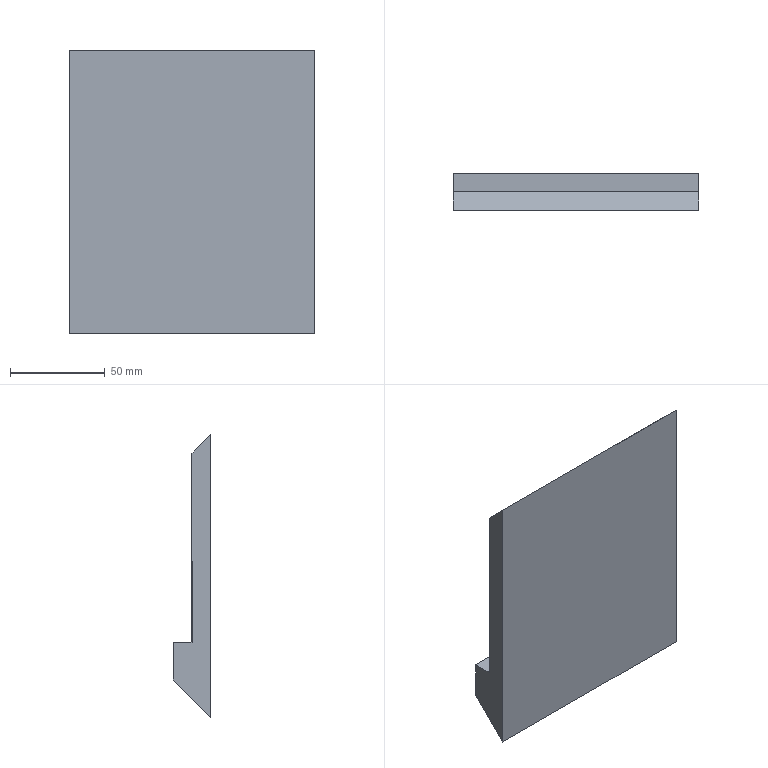Part | NX | features solid 2 | 1 solid | 8 faces | box 130 x 20 x 150 mm | volume 214500 mm3 | plane 8
STEP:
#1=CARTESIAN_POINT('',(830.,185.,120.));
#2=VERTEX_POINT('',#1);
#3=CARTESIAN_POINT('',(700.,185.,120.));
#4=VERTEX_POINT('',#3);
#5=CARTESIAN_POINT('',(695.,185.,120.));
#6=DIRECTION('',(1.,0.,0.));
#7=VECTOR('',#6,1000.);
#8=LINE('',#5,#7);
#9=EDGE_CURVE('',#2,#4,#8,.F.);
#10=ORIENTED_EDGE('',*,*,#9,.F.);
#11=CARTESIAN_POINT('',(830.,185.,20.));
#12=VERTEX_POINT('',#11);
#13=CARTESIAN_POINT('',(830.,185.,10.));
#14=DIRECTION('',(0.,0.,1.));
#15=VECTOR('',#14,1000.);
#16=LINE('',#13,#15);
#17=EDGE_CURVE('',#12,#2,#16,.T.);
#18=ORIENTED_EDGE('',*,*,#17,.F.);
#19=CARTESIAN_POINT('',(700.,185.,20.));
#20=VERTEX_POINT('',#19);
#21=CARTESIAN_POINT('',(730.,185.,20.));
#22=DIRECTION('',(1.,0.,0.));
#23=VECTOR('',#22,1000.);
#24=LINE('',#21,#23);
#25=EDGE_CURVE('',#20,#12,#24,.T.);
#26=ORIENTED_EDGE('',*,*,#25,.F.);
#27=CARTESIAN_POINT('',(700.,185.,95.));
#28=DIRECTION('',(0.,0.,-1.));
#29=VECTOR('',#28,1000.);
#30=LINE('',#27,#29);
#31=EDGE_CURVE('',#4,#20,#30,.T.);
#32=ORIENTED_EDGE('',*,*,#31,.F.);
#33=EDGE_LOOP('',(#10,#18,#26,#32));
#34=FACE_BOUND('',#33,.T.);
#35=CARTESIAN_POINT('',(730.,185.,10.));
#36=DIRECTION('',(0.,1.,0.));
#37=DIRECTION('',(1.,0.,0.));
#38=AXIS2_PLACEMENT_3D('',#35,#36,#37);
#39=PLANE('',#38);
#40=ADVANCED_FACE('',(#34),#39,.T.);
#41=ORIENTED_EDGE('',*,*,#25,.T.);
#42=CARTESIAN_POINT('',(830.,195.,20.));
#43=VERTEX_POINT('',#42);
#44=CARTESIAN_POINT('',(830.,185.,20.));
#45=DIRECTION('',(0.,1.,0.));
#46=VECTOR('',#45,1000.);
#47=LINE('',#44,#46);
#48=EDGE_CURVE('',#43,#12,#47,.F.);
#49=ORIENTED_EDGE('',*,*,#48,.F.);
#50=CARTESIAN_POINT('',(700.,195.,20.));
#51=VERTEX_POINT('',#50);
#52=CARTESIAN_POINT('',(720.,195.,20.));
#53=DIRECTION('',(1.,0.,0.));
#54=VECTOR('',#53,1000.);
#55=LINE('',#52,#54);
#56=EDGE_CURVE('',#51,#43,#55,.T.);
#57=ORIENTED_EDGE('',*,*,#56,.F.);
#58=CARTESIAN_POINT('',(700.,175.,20.));
#59=DIRECTION('',(0.,-1.,0.));
#60=VECTOR('',#59,1000.);
#61=LINE('',#58,#60);
#62=EDGE_CURVE('',#20,#51,#61,.F.);
#63=ORIENTED_EDGE('',*,*,#62,.F.);
#64=EDGE_LOOP('',(#41,#49,#57,#63));
#65=FACE_BOUND('',#64,.T.);
#66=CARTESIAN_POINT('',(720.,175.,20.));
#67=DIRECTION('',(0.,0.,1.));
#68=DIRECTION('',(-1.,0.,0.));
#69=AXIS2_PLACEMENT_3D('',#66,#67,#68);
#70=PLANE('',#69);
#71=ADVANCED_FACE('',(#65),#70,.T.);
#72=ORIENTED_EDGE('',*,*,#56,.T.);
#73=CARTESIAN_POINT('',(830.,195.,0.));
#74=VERTEX_POINT('',#73);
#75=CARTESIAN_POINT('',(830.,195.,20.));
#76=DIRECTION('',(0.,0.,-1.));
#77=VECTOR('',#76,1000.);
#78=LINE('',#75,#77);
#79=EDGE_CURVE('',#74,#43,#78,.F.);
#80=ORIENTED_EDGE('',*,*,#79,.F.);
#81=CARTESIAN_POINT('',(700.,195.,0.));
#82=VERTEX_POINT('',#81);
#83=CARTESIAN_POINT('',(840.,195.,0.));
#84=DIRECTION('',(1.,0.,0.));
#85=VECTOR('',#84,1000.);
#86=LINE('',#83,#85);
#87=EDGE_CURVE('',#82,#74,#86,.T.);
#88=ORIENTED_EDGE('',*,*,#87,.F.);
#89=CARTESIAN_POINT('',(700.,195.,95.));
#90=DIRECTION('',(0.,0.,1.));
#91=VECTOR('',#90,1000.);
#92=LINE('',#89,#91);
#93=EDGE_CURVE('',#51,#82,#92,.F.);
#94=ORIENTED_EDGE('',*,*,#93,.F.);
#95=EDGE_LOOP('',(#72,#80,#88,#94));
#96=FACE_BOUND('',#95,.T.);
#97=CARTESIAN_POINT('',(720.,195.,20.));
#98=DIRECTION('',(0.,-1.,0.));
#99=DIRECTION('',(1.,0.,0.));
#100=AXIS2_PLACEMENT_3D('',#97,#98,#99);
#101=PLANE('',#100);
#102=ADVANCED_FACE('',(#96),#101,.F.);
#103=CARTESIAN_POINT('',(700.,175.,-20.));
#104=VERTEX_POINT('',#103);
#105=CARTESIAN_POINT('',(700.,175.,130.));
#106=VERTEX_POINT('',#105);
#107=CARTESIAN_POINT('',(700.,175.,95.));
#108=DIRECTION('',(0.,0.,-1.));
#109=VECTOR('',#108,1000.);
#110=LINE('',#107,#109);
#111=EDGE_CURVE('',#104,#106,#110,.F.);
#112=ORIENTED_EDGE('',*,*,#111,.F.);
#113=CARTESIAN_POINT('',(830.,175.,-20.));
#114=VERTEX_POINT('',#113);
#115=CARTESIAN_POINT('',(720.,175.,-20.));
#116=DIRECTION('',(-1.,0.,0.));
#117=VECTOR('',#116,1000.);
#118=LINE('',#115,#117);
#119=EDGE_CURVE('',#114,#104,#118,.T.);
#120=ORIENTED_EDGE('',*,*,#119,.F.);
#121=CARTESIAN_POINT('',(830.,175.,130.));
#122=VERTEX_POINT('',#121);
#123=CARTESIAN_POINT('',(830.,175.,130.));
#124=DIRECTION('',(0.,0.,1.));
#125=VECTOR('',#124,1000.);
#126=LINE('',#123,#125);
#127=EDGE_CURVE('',#122,#114,#126,.F.);
#128=ORIENTED_EDGE('',*,*,#127,.F.);
#129=CARTESIAN_POINT('',(830.,175.,130.));
#130=DIRECTION('',(-1.,0.,0.));
#131=VECTOR('',#130,1000.);
#132=LINE('',#129,#131);
#133=EDGE_CURVE('',#106,#122,#132,.F.);
#134=ORIENTED_EDGE('',*,*,#133,.F.);
#135=EDGE_LOOP('',(#112,#120,#128,#134));
#136=FACE_BOUND('',#135,.T.);
#137=CARTESIAN_POINT('',(840.,175.,130.));
#138=DIRECTION('',(0.,1.,0.));
#139=DIRECTION('',(-1.,0.,0.));
#140=AXIS2_PLACEMENT_3D('',#137,#138,#139);
#141=PLANE('',#140);
#142=ADVANCED_FACE('',(#136),#141,.F.);
#143=ORIENTED_EDGE('',*,*,#87,.T.);
#144=CARTESIAN_POINT('',(830.,187.5,-7.5));
#145=DIRECTION('',(0.,-0.7071,-0.7071));
#146=VECTOR('',#145,1000.);
#147=LINE('',#144,#146);
#148=EDGE_CURVE('',#114,#74,#147,.F.);
#149=ORIENTED_EDGE('',*,*,#148,.F.);
#150=ORIENTED_EDGE('',*,*,#119,.T.);
#151=CARTESIAN_POINT('',(700.,195.,0.));
#152=DIRECTION('',(0.,0.7071,0.7071));
#153=VECTOR('',#152,1000.);
#154=LINE('',#151,#153);
#155=EDGE_CURVE('',#82,#104,#154,.F.);
#156=ORIENTED_EDGE('',*,*,#155,.F.);
#157=EDGE_LOOP('',(#143,#149,#150,#156));
#158=FACE_BOUND('',#157,.T.);
#159=CARTESIAN_POINT('',(720.,195.,0.));
#160=DIRECTION('',(0.,0.7071,-0.7071));
#161=DIRECTION('',(0.,0.7071,0.7071));
#162=AXIS2_PLACEMENT_3D('',#159,#160,#161);
#163=PLANE('',#162);
#164=ADVANCED_FACE('',(#158),#163,.T.);
#165=ORIENTED_EDGE('',*,*,#133,.T.);
#166=CARTESIAN_POINT('',(830.,247.5,57.5));
#167=DIRECTION('',(0.,0.7071,-0.7071));
#168=VECTOR('',#167,1000.);
#169=LINE('',#166,#168);
#170=EDGE_CURVE('',#2,#122,#169,.F.);
#171=ORIENTED_EDGE('',*,*,#170,.F.);
#172=ORIENTED_EDGE('',*,*,#9,.T.);
#173=CARTESIAN_POINT('',(700.,185.,120.));
#174=DIRECTION('',(0.,-0.7071,0.7071));
#175=VECTOR('',#174,1000.);
#176=LINE('',#173,#175);
#177=EDGE_CURVE('',#106,#4,#176,.F.);
#178=ORIENTED_EDGE('',*,*,#177,.F.);
#179=EDGE_LOOP('',(#165,#171,#172,#178));
#180=FACE_BOUND('',#179,.T.);
#181=CARTESIAN_POINT('',(730.,185.,120.));
#182=DIRECTION('',(0.,0.7071,0.7071));
#183=DIRECTION('',(0.,0.7071,-0.7071));
#184=AXIS2_PLACEMENT_3D('',#181,#182,#183);
#185=PLANE('',#184);
#186=ADVANCED_FACE('',(#180),#185,.T.);
#187=ORIENTED_EDGE('',*,*,#177,.T.);
#188=ORIENTED_EDGE('',*,*,#31,.T.);
#189=ORIENTED_EDGE('',*,*,#62,.T.);
#190=ORIENTED_EDGE('',*,*,#93,.T.);
#191=ORIENTED_EDGE('',*,*,#155,.T.);
#192=ORIENTED_EDGE('',*,*,#111,.T.);
#193=EDGE_LOOP('',(#187,#188,#189,#190,#191,#192));
#194=FACE_BOUND('',#193,.T.);
#195=CARTESIAN_POINT('',(700.,-355.,95.));
#196=DIRECTION('',(1.,0.,0.));
#197=DIRECTION('',(0.,-1.,0.));
#198=AXIS2_PLACEMENT_3D('',#195,#196,#197);
#199=PLANE('',#198);
#200=ADVANCED_FACE('',(#194),#199,.F.);
#201=ORIENTED_EDGE('',*,*,#148,.T.);
#202=ORIENTED_EDGE('',*,*,#79,.T.);
#203=ORIENTED_EDGE('',*,*,#48,.T.);
#204=ORIENTED_EDGE('',*,*,#17,.T.);
#205=ORIENTED_EDGE('',*,*,#170,.T.);
#206=ORIENTED_EDGE('',*,*,#127,.T.);
#207=EDGE_LOOP('',(#201,#202,#203,#204,#205,#206));
#208=FACE_BOUND('',#207,.T.);
#209=CARTESIAN_POINT('',(830.,185.,-5.));
#210=DIRECTION('',(-1.,0.,0.));
#211=DIRECTION('',(0.,-1.,0.));
#212=AXIS2_PLACEMENT_3D('',#209,#210,#211);
#213=PLANE('',#212);
#214=ADVANCED_FACE('',(#208),#213,.F.);
#215=CLOSED_SHELL('',(#40,#71,#102,#142,#164,#186,#200,#214));
#216=MANIFOLD_SOLID_BREP('',#215);
#217=(LENGTH_UNIT()NAMED_UNIT(*)SI_UNIT(.MILLI.,.METRE.));
#218=UNCERTAINTY_MEASURE_WITH_UNIT(LENGTH_MEASURE(0.00001),#217,'','');
#219=(NAMED_UNIT(*)PLANE_ANGLE_UNIT()SI_UNIT($,.RADIAN.));
#220=(NAMED_UNIT(*)SI_UNIT($,.STERADIAN.)SOLID_ANGLE_UNIT());
#221=(GEOMETRIC_REPRESENTATION_CONTEXT(3)GLOBAL_UNCERTAINTY_ASSIGNED_CONTEXT((#218))GLOBAL_UNIT_ASSIGNED_CONTEXT((#217,#219,#220))REPRESENTATION_CONTEXT('',''));
#222=ADVANCED_BREP_SHAPE_REPRESENTATION('',(#216),#221);